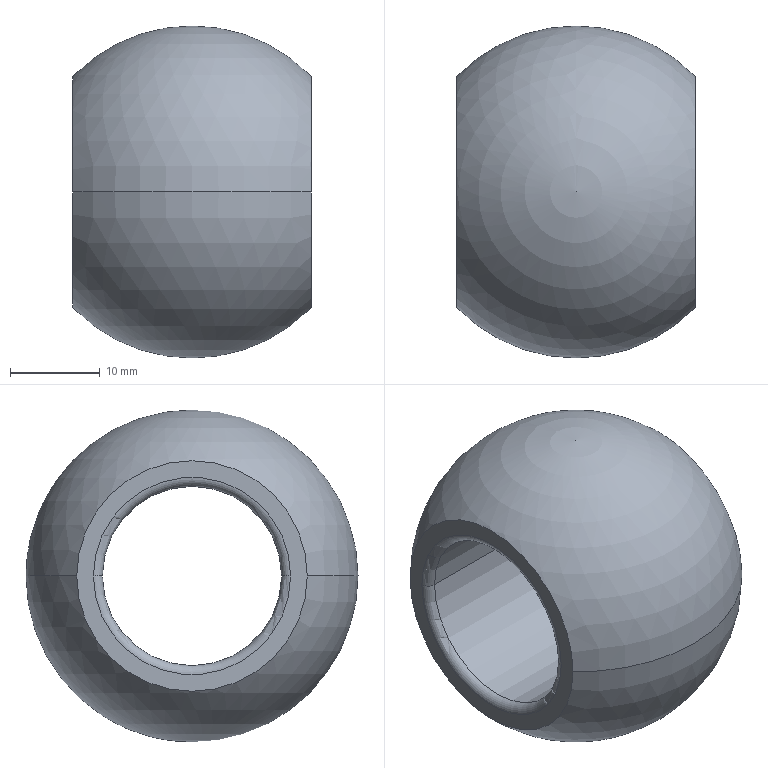Part | STEP file | Rod end bearing | 1 solid | 10 faces | box 26.667 x 37.05 x 37.05 mm | volume 15380 mm3 | torus 4 | sphere 2 | cylinder 2 | plane 2 | commonest cylinder face diameters 20 x2
STEP:
#1=CARTESIAN_POINT('',(13.333,12.861,261.));
#2=VERTEX_POINT('',#1);
#3=CARTESIAN_POINT('',(13.333,-12.861,261.));
#4=VERTEX_POINT('',#3);
#5=CARTESIAN_POINT('',(13.333,0.,261.));
#6=DIRECTION('',(-1.,0.,0.));
#7=DIRECTION('',(0.,-1.,0.));
#8=AXIS2_PLACEMENT_3D('',#5,#6,#7);
#9=CIRCLE('',#8,12.861);
#10=EDGE_CURVE('',#2,#4,#9,.T.);
#11=ORIENTED_EDGE('',*,*,#10,.T.);
#12=CARTESIAN_POINT('',(-13.333,-12.861,261.));
#13=VERTEX_POINT('',#12);
#14=CARTESIAN_POINT('',(0.,0.,261.));
#15=DIRECTION('',(0.,0.,-1.));
#16=DIRECTION('',(0.,1.,0.));
#17=AXIS2_PLACEMENT_3D('',#14,#15,#16);
#18=CIRCLE('',#17,18.525);
#19=EDGE_CURVE('',#4,#13,#18,.T.);
#20=ORIENTED_EDGE('',*,*,#19,.T.);
#21=CARTESIAN_POINT('',(-13.333,12.861,261.));
#22=VERTEX_POINT('',#21);
#23=CARTESIAN_POINT('',(-13.333,0.,261.));
#24=DIRECTION('',(-1.,0.,0.));
#25=DIRECTION('',(0.,-1.,0.));
#26=AXIS2_PLACEMENT_3D('',#23,#24,#25);
#27=CIRCLE('',#26,12.861);
#28=EDGE_CURVE('',#22,#13,#27,.T.);
#29=ORIENTED_EDGE('',*,*,#28,.F.);
#30=CARTESIAN_POINT('',(0.,0.,261.));
#31=DIRECTION('',(0.,0.,1.));
#32=DIRECTION('',(1.,0.,0.));
#33=AXIS2_PLACEMENT_3D('',#30,#31,#32);
#34=CIRCLE('',#33,18.525);
#35=EDGE_CURVE('',#2,#22,#34,.T.);
#36=ORIENTED_EDGE('',*,*,#35,.F.);
#37=EDGE_LOOP('',(#11,#20,#29,#36));
#38=FACE_OUTER_BOUND('',#37,.T.);
#39=CARTESIAN_POINT('',(0.,0.,261.));
#40=DIRECTION('',(0.,0.,-1.));
#41=DIRECTION('',(0.,1.,0.));
#42=AXIS2_PLACEMENT_3D('',#39,#40,#41);
#43=SPHERICAL_SURFACE('',#42,18.525);
#44=ADVANCED_FACE('',(#38),#43,.T.);
#45=CARTESIAN_POINT('',(-13.333,-11.,261.));
#46=VERTEX_POINT('',#45);
#47=CARTESIAN_POINT('',(-13.333,11.,261.));
#48=VERTEX_POINT('',#47);
#49=CARTESIAN_POINT('',(-13.333,0.,261.));
#50=DIRECTION('',(-1.,0.,0.));
#51=DIRECTION('',(0.,-1.,0.));
#52=AXIS2_PLACEMENT_3D('',#49,#50,#51);
#53=CIRCLE('',#52,11.);
#54=EDGE_CURVE('',#46,#48,#53,.T.);
#55=ORIENTED_EDGE('',*,*,#54,.T.);
#56=CARTESIAN_POINT('',(-12.333,10.,261.));
#57=VERTEX_POINT('',#56);
#58=CARTESIAN_POINT('',(-12.333,11.,261.));
#59=DIRECTION('',(0.,0.,1.));
#60=DIRECTION('',(0.,-1.,0.));
#61=AXIS2_PLACEMENT_3D('',#58,#59,#60);
#62=CIRCLE('',#61,1.);
#63=EDGE_CURVE('',#48,#57,#62,.T.);
#64=ORIENTED_EDGE('',*,*,#63,.T.);
#65=CARTESIAN_POINT('',(-12.333,-10.,261.));
#66=VERTEX_POINT('',#65);
#67=CARTESIAN_POINT('',(-12.333,0.,261.));
#68=DIRECTION('',(-1.,0.,0.));
#69=DIRECTION('',(0.,-1.,0.));
#70=AXIS2_PLACEMENT_3D('',#67,#68,#69);
#71=CIRCLE('',#70,10.);
#72=EDGE_CURVE('',#66,#57,#71,.T.);
#73=ORIENTED_EDGE('',*,*,#72,.F.);
#74=CARTESIAN_POINT('',(-12.333,-11.,261.));
#75=DIRECTION('',(0.,0.,-1.));
#76=DIRECTION('',(-1.,0.,0.));
#77=AXIS2_PLACEMENT_3D('',#74,#75,#76);
#78=CIRCLE('',#77,1.);
#79=EDGE_CURVE('',#46,#66,#78,.T.);
#80=ORIENTED_EDGE('',*,*,#79,.F.);
#81=EDGE_LOOP('',(#55,#64,#73,#80));
#82=FACE_OUTER_BOUND('',#81,.T.);
#83=CARTESIAN_POINT('',(-12.333,0.,261.));
#84=DIRECTION('',(-1.,0.,0.));
#85=DIRECTION('',(0.,-1.,0.));
#86=AXIS2_PLACEMENT_3D('',#83,#84,#85);
#87=TOROIDAL_SURFACE('',#86,11.,1.);
#88=ADVANCED_FACE('',(#82),#87,.T.);
#89=CARTESIAN_POINT('',(12.333,10.,261.));
#90=VERTEX_POINT('',#89);
#91=CARTESIAN_POINT('',(12.333,-10.,261.));
#92=VERTEX_POINT('',#91);
#93=CARTESIAN_POINT('',(12.333,0.,261.));
#94=DIRECTION('',(-1.,0.,0.));
#95=DIRECTION('',(0.,-1.,0.));
#96=AXIS2_PLACEMENT_3D('',#93,#94,#95);
#97=CIRCLE('',#96,10.);
#98=EDGE_CURVE('',#90,#92,#97,.T.);
#99=ORIENTED_EDGE('',*,*,#98,.F.);
#100=CARTESIAN_POINT('',(13.333,10.,261.));
#101=DIRECTION('',(-1.,0.,0.));
#102=VECTOR('',#101,1000.);
#103=LINE('',#100,#102);
#104=EDGE_CURVE('',#90,#57,#103,.T.);
#105=ORIENTED_EDGE('',*,*,#104,.T.);
#106=CARTESIAN_POINT('',(-12.333,0.,261.));
#107=DIRECTION('',(-1.,0.,0.));
#108=DIRECTION('',(0.,-1.,0.));
#109=AXIS2_PLACEMENT_3D('',#106,#107,#108);
#110=CIRCLE('',#109,10.);
#111=EDGE_CURVE('',#57,#66,#110,.T.);
#112=ORIENTED_EDGE('',*,*,#111,.T.);
#113=CARTESIAN_POINT('',(13.333,-10.,261.));
#114=DIRECTION('',(-1.,0.,0.));
#115=VECTOR('',#114,1000.);
#116=LINE('',#113,#115);
#117=EDGE_CURVE('',#92,#66,#116,.T.);
#118=ORIENTED_EDGE('',*,*,#117,.F.);
#119=EDGE_LOOP('',(#99,#105,#112,#118));
#120=FACE_OUTER_BOUND('',#119,.T.);
#121=CARTESIAN_POINT('',(13.333,0.,261.));
#122=DIRECTION('',(-1.,0.,0.));
#123=DIRECTION('',(0.,-1.,0.));
#124=AXIS2_PLACEMENT_3D('',#121,#122,#123);
#125=CYLINDRICAL_SURFACE('',#124,10.);
#126=ADVANCED_FACE('',(#120),#125,.F.);
#127=CARTESIAN_POINT('',(12.333,0.,261.));
#128=DIRECTION('',(-1.,0.,0.));
#129=DIRECTION('',(0.,-1.,0.));
#130=AXIS2_PLACEMENT_3D('',#127,#128,#129);
#131=CIRCLE('',#130,10.);
#132=EDGE_CURVE('',#92,#90,#131,.T.);
#133=ORIENTED_EDGE('',*,*,#132,.T.);
#134=CARTESIAN_POINT('',(13.333,11.,261.));
#135=VERTEX_POINT('',#134);
#136=CARTESIAN_POINT('',(12.333,11.,261.));
#137=DIRECTION('',(0.,0.,1.));
#138=DIRECTION('',(0.,-1.,0.));
#139=AXIS2_PLACEMENT_3D('',#136,#137,#138);
#140=CIRCLE('',#139,1.);
#141=EDGE_CURVE('',#90,#135,#140,.T.);
#142=ORIENTED_EDGE('',*,*,#141,.T.);
#143=CARTESIAN_POINT('',(13.333,-11.,261.));
#144=VERTEX_POINT('',#143);
#145=CARTESIAN_POINT('',(13.333,0.,261.));
#146=DIRECTION('',(-1.,0.,0.));
#147=DIRECTION('',(0.,-1.,0.));
#148=AXIS2_PLACEMENT_3D('',#145,#146,#147);
#149=CIRCLE('',#148,11.);
#150=EDGE_CURVE('',#144,#135,#149,.T.);
#151=ORIENTED_EDGE('',*,*,#150,.F.);
#152=CARTESIAN_POINT('',(12.333,-11.,261.));
#153=DIRECTION('',(0.,0.,-1.));
#154=DIRECTION('',(-1.,0.,0.));
#155=AXIS2_PLACEMENT_3D('',#152,#153,#154);
#156=CIRCLE('',#155,1.);
#157=EDGE_CURVE('',#92,#144,#156,.T.);
#158=ORIENTED_EDGE('',*,*,#157,.F.);
#159=EDGE_LOOP('',(#133,#142,#151,#158));
#160=FACE_OUTER_BOUND('',#159,.T.);
#161=CARTESIAN_POINT('',(12.333,0.,261.));
#162=DIRECTION('',(-1.,0.,0.));
#163=DIRECTION('',(0.,-1.,0.));
#164=AXIS2_PLACEMENT_3D('',#161,#162,#163);
#165=TOROIDAL_SURFACE('',#164,11.,1.);
#166=ADVANCED_FACE('',(#160),#165,.T.);
#167=ORIENTED_EDGE('',*,*,#141,.F.);
#168=ORIENTED_EDGE('',*,*,#98,.T.);
#169=ORIENTED_EDGE('',*,*,#157,.T.);
#170=CARTESIAN_POINT('',(13.333,0.,261.));
#171=DIRECTION('',(-1.,0.,0.));
#172=DIRECTION('',(0.,-1.,0.));
#173=AXIS2_PLACEMENT_3D('',#170,#171,#172);
#174=CIRCLE('',#173,11.);
#175=EDGE_CURVE('',#135,#144,#174,.T.);
#176=ORIENTED_EDGE('',*,*,#175,.F.);
#177=EDGE_LOOP('',(#167,#168,#169,#176));
#178=FACE_OUTER_BOUND('',#177,.T.);
#179=CARTESIAN_POINT('',(12.333,0.,261.));
#180=DIRECTION('',(-1.,0.,0.));
#181=DIRECTION('',(0.,-1.,0.));
#182=AXIS2_PLACEMENT_3D('',#179,#180,#181);
#183=TOROIDAL_SURFACE('',#182,11.,1.);
#184=ADVANCED_FACE('',(#178),#183,.T.);
#185=ORIENTED_EDGE('',*,*,#104,.F.);
#186=ORIENTED_EDGE('',*,*,#132,.F.);
#187=ORIENTED_EDGE('',*,*,#117,.T.);
#188=ORIENTED_EDGE('',*,*,#72,.T.);
#189=EDGE_LOOP('',(#185,#186,#187,#188));
#190=FACE_OUTER_BOUND('',#189,.T.);
#191=CARTESIAN_POINT('',(13.333,0.,261.));
#192=DIRECTION('',(-1.,0.,0.));
#193=DIRECTION('',(0.,-1.,0.));
#194=AXIS2_PLACEMENT_3D('',#191,#192,#193);
#195=CYLINDRICAL_SURFACE('',#194,10.);
#196=ADVANCED_FACE('',(#190),#195,.F.);
#197=ORIENTED_EDGE('',*,*,#63,.F.);
#198=CARTESIAN_POINT('',(-13.333,0.,261.));
#199=DIRECTION('',(-1.,0.,0.));
#200=DIRECTION('',(0.,-1.,0.));
#201=AXIS2_PLACEMENT_3D('',#198,#199,#200);
#202=CIRCLE('',#201,11.);
#203=EDGE_CURVE('',#48,#46,#202,.T.);
#204=ORIENTED_EDGE('',*,*,#203,.T.);
#205=ORIENTED_EDGE('',*,*,#79,.T.);
#206=ORIENTED_EDGE('',*,*,#111,.F.);
#207=EDGE_LOOP('',(#197,#204,#205,#206));
#208=FACE_OUTER_BOUND('',#207,.T.);
#209=CARTESIAN_POINT('',(-12.333,0.,261.));
#210=DIRECTION('',(-1.,0.,0.));
#211=DIRECTION('',(0.,-1.,0.));
#212=AXIS2_PLACEMENT_3D('',#209,#210,#211);
#213=TOROIDAL_SURFACE('',#212,11.,1.);
#214=ADVANCED_FACE('',(#208),#213,.T.);
#215=ORIENTED_EDGE('',*,*,#28,.T.);
#216=CARTESIAN_POINT('',(-13.333,0.,261.));
#217=DIRECTION('',(-1.,0.,0.));
#218=DIRECTION('',(0.,-1.,0.));
#219=AXIS2_PLACEMENT_3D('',#216,#217,#218);
#220=CIRCLE('',#219,12.861);
#221=EDGE_CURVE('',#13,#22,#220,.T.);
#222=ORIENTED_EDGE('',*,*,#221,.T.);
#223=EDGE_LOOP('',(#215,#222));
#224=FACE_OUTER_BOUND('',#223,.T.);
#225=ORIENTED_EDGE('',*,*,#54,.F.);
#226=ORIENTED_EDGE('',*,*,#203,.F.);
#227=EDGE_LOOP('',(#225,#226));
#228=FACE_BOUND('',#227,.T.);
#229=CARTESIAN_POINT('',(-13.333,11.,261.));
#230=DIRECTION('',(-1.,0.,0.));
#231=DIRECTION('',(0.,-1.,0.));
#232=AXIS2_PLACEMENT_3D('',#229,#230,#231);
#233=PLANE('',#232);
#234=ADVANCED_FACE('',(#224,#228),#233,.T.);
#235=ORIENTED_EDGE('',*,*,#19,.F.);
#236=CARTESIAN_POINT('',(13.333,0.,261.));
#237=DIRECTION('',(-1.,0.,0.));
#238=DIRECTION('',(0.,-1.,0.));
#239=AXIS2_PLACEMENT_3D('',#236,#237,#238);
#240=CIRCLE('',#239,12.861);
#241=EDGE_CURVE('',#4,#2,#240,.T.);
#242=ORIENTED_EDGE('',*,*,#241,.T.);
#243=ORIENTED_EDGE('',*,*,#35,.T.);
#244=ORIENTED_EDGE('',*,*,#221,.F.);
#245=EDGE_LOOP('',(#235,#242,#243,#244));
#246=FACE_OUTER_BOUND('',#245,.T.);
#247=CARTESIAN_POINT('',(0.,0.,261.));
#248=DIRECTION('',(0.,0.,-1.));
#249=DIRECTION('',(0.,1.,0.));
#250=AXIS2_PLACEMENT_3D('',#247,#248,#249);
#251=SPHERICAL_SURFACE('',#250,18.525);
#252=ADVANCED_FACE('',(#246),#251,.T.);
#253=ORIENTED_EDGE('',*,*,#150,.T.);
#254=ORIENTED_EDGE('',*,*,#175,.T.);
#255=EDGE_LOOP('',(#253,#254));
#256=FACE_BOUND('',#255,.T.);
#257=ORIENTED_EDGE('',*,*,#10,.F.);
#258=ORIENTED_EDGE('',*,*,#241,.F.);
#259=EDGE_LOOP('',(#257,#258));
#260=FACE_OUTER_BOUND('',#259,.T.);
#261=CARTESIAN_POINT('',(13.333,12.861,261.));
#262=DIRECTION('',(1.,0.,0.));
#263=DIRECTION('',(0.,1.,0.));
#264=AXIS2_PLACEMENT_3D('',#261,#262,#263);
#265=PLANE('',#264);
#266=ADVANCED_FACE('',(#256,#260),#265,.T.);
#267=CLOSED_SHELL('',(#44,#88,#126,#166,#184,#196,#214,#234,#252,#266));
#268=MANIFOLD_SOLID_BREP('',#267);
#269=CARTESIAN_POINT('',(0.,0.,0.));
#270=DIRECTION('',(0.,0.,1.));
#271=DIRECTION('',(1.,0.,0.));
#272=AXIS2_PLACEMENT_3D('',#269,#270,#271);
#273=(LENGTH_UNIT()NAMED_UNIT(*)SI_UNIT(.MILLI.,.METRE.));
#274=UNCERTAINTY_MEASURE_WITH_UNIT(LENGTH_MEASURE(0.00001),#273,'','');
#275=(NAMED_UNIT(*)PLANE_ANGLE_UNIT()SI_UNIT($,.RADIAN.));
#276=(NAMED_UNIT(*)SI_UNIT($,.STERADIAN.)SOLID_ANGLE_UNIT());
#277=(GEOMETRIC_REPRESENTATION_CONTEXT(3)GLOBAL_UNCERTAINTY_ASSIGNED_CONTEXT((#274))GLOBAL_UNIT_ASSIGNED_CONTEXT((#273,#275,#276))REPRESENTATION_CONTEXT('',''));
#278=ADVANCED_BREP_SHAPE_REPRESENTATION('',(#268,#272),#277);